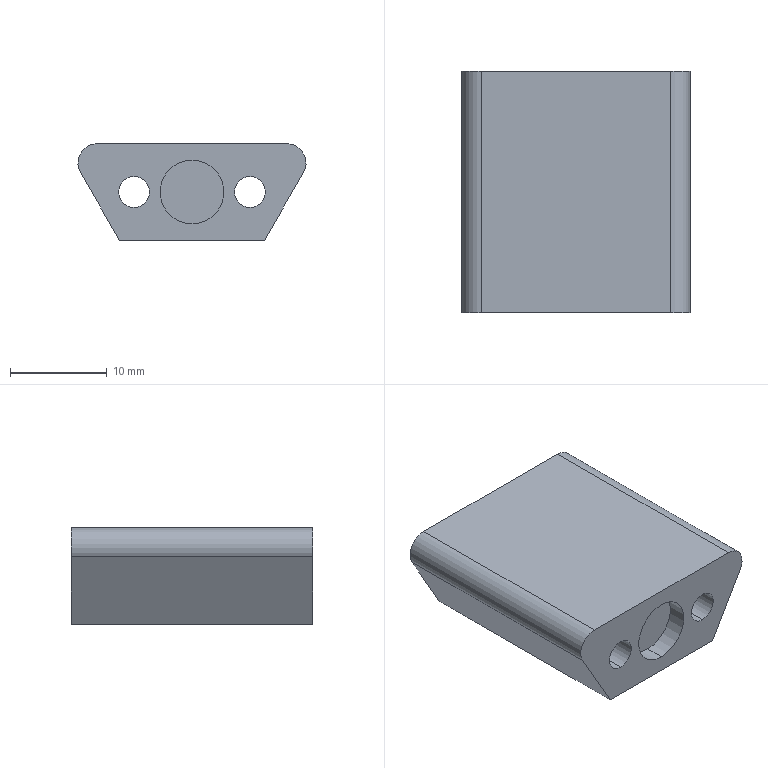Part | SolidWorks | features HoleWzd 2, ICE 2, Extrusion 1 | 1 solid | 29 faces | box 23.619 x 25 x 10 mm | volume 4394 mm3 | cylinder 16 | plane 9 | cone 4 | commonest cylinder face diameters 2.5 x4 3.2 x4 5 x4 4 x2 6.6 x2
STEP:
#1=CARTESIAN_POINT('',(13.274,-10.5,-1.7));
#2=VERTEX_POINT('',#1);
#3=CARTESIAN_POINT('',(13.274,-10.5,-8.3));
#4=VERTEX_POINT('',#3);
#5=CARTESIAN_POINT('',(13.274,-10.5,-5.));
#6=DIRECTION('',(0.,-1.,0.));
#7=DIRECTION('',(0.,0.,-1.));
#8=AXIS2_PLACEMENT_3D('',#5,#6,#7);
#9=CIRCLE('',#8,3.3);
#10=EDGE_CURVE('',#2,#4,#9,.T.);
#11=ORIENTED_EDGE('',*,*,#10,.F.);
#12=CARTESIAN_POINT('',(13.274,-12.5,-1.7));
#13=VERTEX_POINT('',#12);
#14=CARTESIAN_POINT('',(13.274,-10.5,-1.7));
#15=DIRECTION('',(0.,-1.,0.));
#16=VECTOR('',#15,1000.);
#17=LINE('',#14,#16);
#18=EDGE_CURVE('',#2,#13,#17,.T.);
#19=ORIENTED_EDGE('',*,*,#18,.T.);
#20=CARTESIAN_POINT('',(13.274,-12.5,-8.3));
#21=VERTEX_POINT('',#20);
#22=CARTESIAN_POINT('',(13.274,-12.5,-5.));
#23=DIRECTION('',(0.,-1.,0.));
#24=DIRECTION('',(0.,0.,-1.));
#25=AXIS2_PLACEMENT_3D('',#22,#23,#24);
#26=CIRCLE('',#25,3.3);
#27=EDGE_CURVE('',#13,#21,#26,.T.);
#28=ORIENTED_EDGE('',*,*,#27,.T.);
#29=CARTESIAN_POINT('',(13.274,-10.5,-8.3));
#30=DIRECTION('',(0.,-1.,0.));
#31=VECTOR('',#30,1000.);
#32=LINE('',#29,#31);
#33=EDGE_CURVE('',#4,#21,#32,.T.);
#34=ORIENTED_EDGE('',*,*,#33,.F.);
#35=EDGE_LOOP('',(#11,#19,#28,#34));
#36=FACE_OUTER_BOUND('',#35,.T.);
#37=CARTESIAN_POINT('',(13.274,-10.5,-5.));
#38=DIRECTION('',(0.,-1.,0.));
#39=DIRECTION('',(0.,0.,-1.));
#40=AXIS2_PLACEMENT_3D('',#37,#38,#39);
#41=CYLINDRICAL_SURFACE('',#40,3.3);
#42=ADVANCED_FACE('',(#36),#41,.F.);
#43=CARTESIAN_POINT('',(19.274,-12.5,-6.6));
#44=VERTEX_POINT('',#43);
#45=CARTESIAN_POINT('',(19.274,-12.5,-3.4));
#46=VERTEX_POINT('',#45);
#47=CARTESIAN_POINT('',(19.274,-12.5,-5.));
#48=DIRECTION('',(0.,1.,0.));
#49=DIRECTION('',(0.,0.,1.));
#50=AXIS2_PLACEMENT_3D('',#47,#48,#49);
#51=CIRCLE('',#50,1.6);
#52=EDGE_CURVE('',#44,#46,#51,.T.);
#53=ORIENTED_EDGE('',*,*,#52,.F.);
#54=CARTESIAN_POINT('',(19.274,7.5,-6.6));
#55=VERTEX_POINT('',#54);
#56=CARTESIAN_POINT('',(19.274,7.5,-6.6));
#57=DIRECTION('',(0.,1.,0.));
#58=VECTOR('',#57,1000.);
#59=LINE('',#56,#58);
#60=EDGE_CURVE('',#44,#55,#59,.T.);
#61=ORIENTED_EDGE('',*,*,#60,.T.);
#62=CARTESIAN_POINT('',(19.274,7.5,-3.4));
#63=VERTEX_POINT('',#62);
#64=CARTESIAN_POINT('',(19.274,7.5,-5.));
#65=DIRECTION('',(0.,1.,0.));
#66=DIRECTION('',(0.,0.,1.));
#67=AXIS2_PLACEMENT_3D('',#64,#65,#66);
#68=CIRCLE('',#67,1.6);
#69=EDGE_CURVE('',#55,#63,#68,.T.);
#70=ORIENTED_EDGE('',*,*,#69,.T.);
#71=CARTESIAN_POINT('',(19.274,7.5,-3.4));
#72=DIRECTION('',(0.,1.,0.));
#73=VECTOR('',#72,1000.);
#74=LINE('',#71,#73);
#75=EDGE_CURVE('',#46,#63,#74,.T.);
#76=ORIENTED_EDGE('',*,*,#75,.F.);
#77=EDGE_LOOP('',(#53,#61,#70,#76));
#78=FACE_OUTER_BOUND('',#77,.T.);
#79=CARTESIAN_POINT('',(19.274,7.5,-5.));
#80=DIRECTION('',(0.,1.,0.));
#81=DIRECTION('',(0.,0.,1.));
#82=AXIS2_PLACEMENT_3D('',#79,#80,#81);
#83=CYLINDRICAL_SURFACE('',#82,1.6);
#84=ADVANCED_FACE('',(#78),#83,.F.);
#85=CARTESIAN_POINT('',(7.274,-12.5,-6.6));
#86=VERTEX_POINT('',#85);
#87=CARTESIAN_POINT('',(7.274,-12.5,-3.4));
#88=VERTEX_POINT('',#87);
#89=CARTESIAN_POINT('',(7.274,-12.5,-5.));
#90=DIRECTION('',(0.,1.,0.));
#91=DIRECTION('',(0.,0.,1.));
#92=AXIS2_PLACEMENT_3D('',#89,#90,#91);
#93=CIRCLE('',#92,1.6);
#94=EDGE_CURVE('',#86,#88,#93,.T.);
#95=ORIENTED_EDGE('',*,*,#94,.F.);
#96=CARTESIAN_POINT('',(7.274,7.5,-6.6));
#97=VERTEX_POINT('',#96);
#98=CARTESIAN_POINT('',(7.274,7.5,-6.6));
#99=DIRECTION('',(0.,1.,0.));
#100=VECTOR('',#99,1000.);
#101=LINE('',#98,#100);
#102=EDGE_CURVE('',#86,#97,#101,.T.);
#103=ORIENTED_EDGE('',*,*,#102,.T.);
#104=CARTESIAN_POINT('',(7.274,7.5,-3.4));
#105=VERTEX_POINT('',#104);
#106=CARTESIAN_POINT('',(7.274,7.5,-5.));
#107=DIRECTION('',(0.,1.,0.));
#108=DIRECTION('',(0.,0.,1.));
#109=AXIS2_PLACEMENT_3D('',#106,#107,#108);
#110=CIRCLE('',#109,1.6);
#111=EDGE_CURVE('',#97,#105,#110,.T.);
#112=ORIENTED_EDGE('',*,*,#111,.T.);
#113=CARTESIAN_POINT('',(7.274,7.5,-3.4));
#114=DIRECTION('',(0.,1.,0.));
#115=VECTOR('',#114,1000.);
#116=LINE('',#113,#115);
#117=EDGE_CURVE('',#88,#105,#116,.T.);
#118=ORIENTED_EDGE('',*,*,#117,.F.);
#119=EDGE_LOOP('',(#95,#103,#112,#118));
#120=FACE_OUTER_BOUND('',#119,.T.);
#121=CARTESIAN_POINT('',(7.274,7.5,-5.));
#122=DIRECTION('',(0.,1.,0.));
#123=DIRECTION('',(0.,0.,1.));
#124=AXIS2_PLACEMENT_3D('',#121,#122,#123);
#125=CYLINDRICAL_SURFACE('',#124,1.6);
#126=ADVANCED_FACE('',(#120),#125,.F.);
#127=CARTESIAN_POINT('',(14.524,-5.,-2.5));
#128=VERTEX_POINT('',#127);
#129=CARTESIAN_POINT('',(12.024,-5.,-2.5));
#130=VERTEX_POINT('',#129);
#131=CARTESIAN_POINT('',(13.274,-5.,-2.5));
#132=DIRECTION('',(0.,0.,-1.));
#133=DIRECTION('',(-1.,0.,0.));
#134=AXIS2_PLACEMENT_3D('',#131,#132,#133);
#135=CIRCLE('',#134,1.25);
#136=EDGE_CURVE('',#128,#130,#135,.T.);
#137=ORIENTED_EDGE('',*,*,#136,.F.);
#138=CARTESIAN_POINT('',(14.524,-5.,-10.));
#139=VERTEX_POINT('',#138);
#140=CARTESIAN_POINT('',(14.524,-5.,-10.));
#141=DIRECTION('',(0.,0.,-1.));
#142=VECTOR('',#141,1000.);
#143=LINE('',#140,#142);
#144=EDGE_CURVE('',#128,#139,#143,.T.);
#145=ORIENTED_EDGE('',*,*,#144,.T.);
#146=CARTESIAN_POINT('',(12.024,-5.,-10.));
#147=VERTEX_POINT('',#146);
#148=CARTESIAN_POINT('',(13.274,-5.,-10.));
#149=DIRECTION('',(0.,0.,-1.));
#150=DIRECTION('',(-1.,0.,0.));
#151=AXIS2_PLACEMENT_3D('',#148,#149,#150);
#152=CIRCLE('',#151,1.25);
#153=EDGE_CURVE('',#139,#147,#152,.T.);
#154=ORIENTED_EDGE('',*,*,#153,.T.);
#155=CARTESIAN_POINT('',(12.024,-5.,-10.));
#156=DIRECTION('',(0.,0.,-1.));
#157=VECTOR('',#156,1000.);
#158=LINE('',#155,#157);
#159=EDGE_CURVE('',#130,#147,#158,.T.);
#160=ORIENTED_EDGE('',*,*,#159,.F.);
#161=EDGE_LOOP('',(#137,#145,#154,#160));
#162=FACE_OUTER_BOUND('',#161,.T.);
#163=CARTESIAN_POINT('',(13.274,-5.,-10.));
#164=DIRECTION('',(0.,0.,-1.));
#165=DIRECTION('',(-1.,0.,0.));
#166=AXIS2_PLACEMENT_3D('',#163,#164,#165);
#167=CYLINDRICAL_SURFACE('',#166,1.25);
#168=ADVANCED_FACE('',(#162),#167,.F.);
#169=CARTESIAN_POINT('',(13.274,-5.,-1.749));
#170=VERTEX_POINT('',#169);
#171=CARTESIAN_POINT('',(12.024,-5.,-2.5));
#172=DIRECTION('',(-0.8572,0.,-0.515));
#173=VECTOR('',#172,1000.);
#174=LINE('',#171,#173);
#175=EDGE_CURVE('',#170,#130,#174,.T.);
#176=ORIENTED_EDGE('',*,*,#175,.F.);
#177=CARTESIAN_POINT('',(14.524,-5.,-2.5));
#178=DIRECTION('',(0.8572,0.,-0.515));
#179=VECTOR('',#178,1000.);
#180=LINE('',#177,#179);
#181=EDGE_CURVE('',#170,#128,#180,.T.);
#182=ORIENTED_EDGE('',*,*,#181,.T.);
#183=ORIENTED_EDGE('',*,*,#136,.T.);
#184=EDGE_LOOP('',(#176,#182,#183));
#185=FACE_OUTER_BOUND('',#184,.T.);
#186=CARTESIAN_POINT('',(13.274,-5.,-2.5));
#187=DIRECTION('',(0.,0.,-1.));
#188=DIRECTION('',(-1.,0.,0.));
#189=AXIS2_PLACEMENT_3D('',#186,#187,#188);
#190=CONICAL_SURFACE('',#189,1.25,1.03);
#191=ADVANCED_FACE('',(#185),#190,.F.);
#192=CARTESIAN_POINT('',(14.524,5.,-2.5));
#193=VERTEX_POINT('',#192);
#194=CARTESIAN_POINT('',(12.024,5.,-2.5));
#195=VERTEX_POINT('',#194);
#196=CARTESIAN_POINT('',(13.274,5.,-2.5));
#197=DIRECTION('',(0.,0.,-1.));
#198=DIRECTION('',(-1.,0.,0.));
#199=AXIS2_PLACEMENT_3D('',#196,#197,#198);
#200=CIRCLE('',#199,1.25);
#201=EDGE_CURVE('',#193,#195,#200,.T.);
#202=ORIENTED_EDGE('',*,*,#201,.F.);
#203=CARTESIAN_POINT('',(14.524,5.,-10.));
#204=VERTEX_POINT('',#203);
#205=CARTESIAN_POINT('',(14.524,5.,-10.));
#206=DIRECTION('',(0.,0.,-1.));
#207=VECTOR('',#206,1000.);
#208=LINE('',#205,#207);
#209=EDGE_CURVE('',#193,#204,#208,.T.);
#210=ORIENTED_EDGE('',*,*,#209,.T.);
#211=CARTESIAN_POINT('',(12.024,5.,-10.));
#212=VERTEX_POINT('',#211);
#213=CARTESIAN_POINT('',(13.274,5.,-10.));
#214=DIRECTION('',(0.,0.,-1.));
#215=DIRECTION('',(-1.,0.,0.));
#216=AXIS2_PLACEMENT_3D('',#213,#214,#215);
#217=CIRCLE('',#216,1.25);
#218=EDGE_CURVE('',#204,#212,#217,.T.);
#219=ORIENTED_EDGE('',*,*,#218,.T.);
#220=CARTESIAN_POINT('',(12.024,5.,-10.));
#221=DIRECTION('',(0.,0.,-1.));
#222=VECTOR('',#221,1000.);
#223=LINE('',#220,#222);
#224=EDGE_CURVE('',#195,#212,#223,.T.);
#225=ORIENTED_EDGE('',*,*,#224,.F.);
#226=EDGE_LOOP('',(#202,#210,#219,#225));
#227=FACE_OUTER_BOUND('',#226,.T.);
#228=CARTESIAN_POINT('',(13.274,5.,-10.));
#229=DIRECTION('',(0.,0.,-1.));
#230=DIRECTION('',(-1.,0.,0.));
#231=AXIS2_PLACEMENT_3D('',#228,#229,#230);
#232=CYLINDRICAL_SURFACE('',#231,1.25);
#233=ADVANCED_FACE('',(#227),#232,.F.);
#234=CARTESIAN_POINT('',(13.274,5.,-1.749));
#235=VERTEX_POINT('',#234);
#236=CARTESIAN_POINT('',(12.024,5.,-2.5));
#237=DIRECTION('',(-0.8572,0.,-0.515));
#238=VECTOR('',#237,1000.);
#239=LINE('',#236,#238);
#240=EDGE_CURVE('',#235,#195,#239,.T.);
#241=ORIENTED_EDGE('',*,*,#240,.F.);
#242=CARTESIAN_POINT('',(14.524,5.,-2.5));
#243=DIRECTION('',(0.8572,0.,-0.515));
#244=VECTOR('',#243,1000.);
#245=LINE('',#242,#244);
#246=EDGE_CURVE('',#235,#193,#245,.T.);
#247=ORIENTED_EDGE('',*,*,#246,.T.);
#248=ORIENTED_EDGE('',*,*,#201,.T.);
#249=EDGE_LOOP('',(#241,#247,#248));
#250=FACE_OUTER_BOUND('',#249,.T.);
#251=CARTESIAN_POINT('',(13.274,5.,-2.5));
#252=DIRECTION('',(0.,0.,-1.));
#253=DIRECTION('',(-1.,0.,0.));
#254=AXIS2_PLACEMENT_3D('',#251,#252,#253);
#255=CONICAL_SURFACE('',#254,1.25,1.03);
#256=ADVANCED_FACE('',(#250),#255,.F.);
#257=CARTESIAN_POINT('',(19.274,7.5,-7.5));
#258=VERTEX_POINT('',#257);
#259=CARTESIAN_POINT('',(19.274,7.5,-2.5));
#260=VERTEX_POINT('',#259);
#261=CARTESIAN_POINT('',(19.274,7.5,-5.));
#262=DIRECTION('',(0.,1.,0.));
#263=DIRECTION('',(0.,0.,1.));
#264=AXIS2_PLACEMENT_3D('',#261,#262,#263);
#265=CIRCLE('',#264,2.5);
#266=EDGE_CURVE('',#258,#260,#265,.T.);
#267=ORIENTED_EDGE('',*,*,#266,.F.);
#268=CARTESIAN_POINT('',(19.274,12.5,-7.5));
#269=VERTEX_POINT('',#268);
#270=CARTESIAN_POINT('',(19.274,7.5,-7.5));
#271=DIRECTION('',(0.,1.,0.));
#272=VECTOR('',#271,1000.);
#273=LINE('',#270,#272);
#274=EDGE_CURVE('',#258,#269,#273,.T.);
#275=ORIENTED_EDGE('',*,*,#274,.T.);
#276=CARTESIAN_POINT('',(19.274,12.5,-2.5));
#277=VERTEX_POINT('',#276);
#278=CARTESIAN_POINT('',(19.274,12.5,-5.));
#279=DIRECTION('',(0.,1.,0.));
#280=DIRECTION('',(0.,0.,1.));
#281=AXIS2_PLACEMENT_3D('',#278,#279,#280);
#282=CIRCLE('',#281,2.5);
#283=EDGE_CURVE('',#269,#277,#282,.T.);
#284=ORIENTED_EDGE('',*,*,#283,.T.);
#285=CARTESIAN_POINT('',(19.274,7.5,-2.5));
#286=DIRECTION('',(0.,1.,0.));
#287=VECTOR('',#286,1000.);
#288=LINE('',#285,#287);
#289=EDGE_CURVE('',#260,#277,#288,.T.);
#290=ORIENTED_EDGE('',*,*,#289,.F.);
#291=EDGE_LOOP('',(#267,#275,#284,#290));
#292=FACE_OUTER_BOUND('',#291,.T.);
#293=CARTESIAN_POINT('',(19.274,7.5,-5.));
#294=DIRECTION('',(0.,1.,0.));
#295=DIRECTION('',(0.,0.,1.));
#296=AXIS2_PLACEMENT_3D('',#293,#294,#295);
#297=CYLINDRICAL_SURFACE('',#296,2.5);
#298=ADVANCED_FACE('',(#292),#297,.F.);
#299=CARTESIAN_POINT('',(7.274,7.5,-7.5));
#300=VERTEX_POINT('',#299);
#301=CARTESIAN_POINT('',(7.274,7.5,-2.5));
#302=VERTEX_POINT('',#301);
#303=CARTESIAN_POINT('',(7.274,7.5,-5.));
#304=DIRECTION('',(0.,1.,0.));
#305=DIRECTION('',(0.,0.,1.));
#306=AXIS2_PLACEMENT_3D('',#303,#304,#305);
#307=CIRCLE('',#306,2.5);
#308=EDGE_CURVE('',#300,#302,#307,.T.);
#309=ORIENTED_EDGE('',*,*,#308,.F.);
#310=CARTESIAN_POINT('',(7.274,12.5,-7.5));
#311=VERTEX_POINT('',#310);
#312=CARTESIAN_POINT('',(7.274,7.5,-7.5));
#313=DIRECTION('',(0.,1.,0.));
#314=VECTOR('',#313,1000.);
#315=LINE('',#312,#314);
#316=EDGE_CURVE('',#300,#311,#315,.T.);
#317=ORIENTED_EDGE('',*,*,#316,.T.);
#318=CARTESIAN_POINT('',(7.274,12.5,-2.5));
#319=VERTEX_POINT('',#318);
#320=CARTESIAN_POINT('',(7.274,12.5,-5.));
#321=DIRECTION('',(0.,1.,0.));
#322=DIRECTION('',(0.,0.,1.));
#323=AXIS2_PLACEMENT_3D('',#320,#321,#322);
#324=CIRCLE('',#323,2.5);
#325=EDGE_CURVE('',#311,#319,#324,.T.);
#326=ORIENTED_EDGE('',*,*,#325,.T.);
#327=CARTESIAN_POINT('',(7.274,7.5,-2.5));
#328=DIRECTION('',(0.,1.,0.));
#329=VECTOR('',#328,1000.);
#330=LINE('',#327,#329);
#331=EDGE_CURVE('',#302,#319,#330,.T.);
#332=ORIENTED_EDGE('',*,*,#331,.F.);
#333=EDGE_LOOP('',(#309,#317,#326,#332));
#334=FACE_OUTER_BOUND('',#333,.T.);
#335=CARTESIAN_POINT('',(7.274,7.5,-5.));
#336=DIRECTION('',(0.,1.,0.));
#337=DIRECTION('',(0.,0.,1.));
#338=AXIS2_PLACEMENT_3D('',#335,#336,#337);
#339=CYLINDRICAL_SURFACE('',#338,2.5);
#340=ADVANCED_FACE('',(#334),#339,.F.);
#341=CARTESIAN_POINT('',(13.274,-5.,-10.));
#342=DIRECTION('',(0.,0.,-1.));
#343=DIRECTION('',(-1.,0.,0.));
#344=AXIS2_PLACEMENT_3D('',#341,#342,#343);
#345=CIRCLE('',#344,1.25);
#346=EDGE_CURVE('',#147,#139,#345,.T.);
#347=ORIENTED_EDGE('',*,*,#346,.F.);
#348=ORIENTED_EDGE('',*,*,#153,.F.);
#349=EDGE_LOOP('',(#347,#348));
#350=FACE_BOUND('',#349,.T.);
#351=CARTESIAN_POINT('',(13.274,5.,-10.));
#352=DIRECTION('',(0.,0.,-1.));
#353=DIRECTION('',(-1.,0.,0.));
#354=AXIS2_PLACEMENT_3D('',#351,#352,#353);
#355=CIRCLE('',#354,1.25);
#356=EDGE_CURVE('',#212,#204,#355,.T.);
#357=ORIENTED_EDGE('',*,*,#356,.F.);
#358=ORIENTED_EDGE('',*,*,#218,.F.);
#359=EDGE_LOOP('',(#357,#358));
#360=FACE_BOUND('',#359,.T.);
#361=CARTESIAN_POINT('',(20.774,-12.5,-10.));
#362=VERTEX_POINT('',#361);
#363=CARTESIAN_POINT('',(5.774,-12.5,-10.));
#364=VERTEX_POINT('',#363);
#365=CARTESIAN_POINT('',(20.774,-12.5,-10.));
#366=DIRECTION('',(-1.,0.,0.));
#367=VECTOR('',#366,1000.);
#368=LINE('',#365,#367);
#369=EDGE_CURVE('',#362,#364,#368,.T.);
#370=ORIENTED_EDGE('',*,*,#369,.T.);
#371=CARTESIAN_POINT('',(5.774,12.5,-10.));
#372=VERTEX_POINT('',#371);
#373=CARTESIAN_POINT('',(5.774,12.5,-10.));
#374=DIRECTION('',(0.,-1.,0.));
#375=VECTOR('',#374,1000.);
#376=LINE('',#373,#375);
#377=EDGE_CURVE('',#372,#364,#376,.T.);
#378=ORIENTED_EDGE('',*,*,#377,.F.);
#379=CARTESIAN_POINT('',(20.774,12.5,-10.));
#380=VERTEX_POINT('',#379);
#381=CARTESIAN_POINT('',(20.774,12.5,-10.));
#382=DIRECTION('',(-1.,0.,0.));
#383=VECTOR('',#382,1000.);
#384=LINE('',#381,#383);
#385=EDGE_CURVE('',#380,#372,#384,.T.);
#386=ORIENTED_EDGE('',*,*,#385,.F.);
#387=CARTESIAN_POINT('',(20.774,12.5,-10.));
#388=DIRECTION('',(0.,-1.,0.));
#389=VECTOR('',#388,1000.);
#390=LINE('',#387,#389);
#391=EDGE_CURVE('',#380,#362,#390,.T.);
#392=ORIENTED_EDGE('',*,*,#391,.T.);
#393=EDGE_LOOP('',(#370,#378,#386,#392));
#394=FACE_OUTER_BOUND('',#393,.T.);
#395=CARTESIAN_POINT('',(20.774,12.5,-10.));
#396=DIRECTION('',(0.,0.,1.));
#397=DIRECTION('',(1.,0.,0.));
#398=AXIS2_PLACEMENT_3D('',#395,#396,#397);
#399=PLANE('',#398);
#400=ADVANCED_FACE('',(#350,#360,#394),#399,.F.);
#401=CARTESIAN_POINT('',(1.732,-12.5,-3.));
#402=VERTEX_POINT('',#401);
#403=CARTESIAN_POINT('',(5.774,-12.5,-10.));
#404=DIRECTION('',(-0.5,0.,0.866));
#405=VECTOR('',#404,1000.);
#406=LINE('',#403,#405);
#407=EDGE_CURVE('',#364,#402,#406,.T.);
#408=ORIENTED_EDGE('',*,*,#407,.T.);
#409=CARTESIAN_POINT('',(1.732,12.5,-3.));
#410=VERTEX_POINT('',#409);
#411=CARTESIAN_POINT('',(1.732,12.5,-3.));
#412=DIRECTION('',(0.,-1.,0.));
#413=VECTOR('',#412,1000.);
#414=LINE('',#411,#413);
#415=EDGE_CURVE('',#410,#402,#414,.T.);
#416=ORIENTED_EDGE('',*,*,#415,.F.);
#417=CARTESIAN_POINT('',(5.774,12.5,-10.));
#418=DIRECTION('',(-0.5,0.,0.866));
#419=VECTOR('',#418,1000.);
#420=LINE('',#417,#419);
#421=EDGE_CURVE('',#372,#410,#420,.T.);
#422=ORIENTED_EDGE('',*,*,#421,.F.);
#423=ORIENTED_EDGE('',*,*,#377,.T.);
#424=EDGE_LOOP('',(#408,#416,#422,#423));
#425=FACE_OUTER_BOUND('',#424,.T.);
#426=CARTESIAN_POINT('',(5.774,12.5,-10.));
#427=DIRECTION('',(0.866,0.,0.5));
#428=DIRECTION('',(0.5,0.,-0.866));
#429=AXIS2_PLACEMENT_3D('',#426,#427,#428);
#430=PLANE('',#429);
#431=ADVANCED_FACE('',(#425),#430,.F.);
#432=CARTESIAN_POINT('',(3.464,-12.5,0.));
#433=VERTEX_POINT('',#432);
#434=CARTESIAN_POINT('',(3.464,-12.5,-2.));
#435=DIRECTION('',(0.,1.,0.));
#436=DIRECTION('',(0.,0.,-1.));
#437=AXIS2_PLACEMENT_3D('',#434,#435,#436);
#438=CIRCLE('',#437,2.);
#439=EDGE_CURVE('',#402,#433,#438,.T.);
#440=ORIENTED_EDGE('',*,*,#439,.T.);
#441=CARTESIAN_POINT('',(3.464,12.5,0.));
#442=VERTEX_POINT('',#441);
#443=CARTESIAN_POINT('',(3.464,12.5,0.));
#444=DIRECTION('',(0.,-1.,0.));
#445=VECTOR('',#444,1000.);
#446=LINE('',#443,#445);
#447=EDGE_CURVE('',#442,#433,#446,.T.);
#448=ORIENTED_EDGE('',*,*,#447,.F.);
#449=CARTESIAN_POINT('',(3.464,12.5,-2.));
#450=DIRECTION('',(0.,1.,0.));
#451=DIRECTION('',(0.,0.,-1.));
#452=AXIS2_PLACEMENT_3D('',#449,#450,#451);
#453=CIRCLE('',#452,2.);
#454=EDGE_CURVE('',#410,#442,#453,.T.);
#455=ORIENTED_EDGE('',*,*,#454,.F.);
#456=ORIENTED_EDGE('',*,*,#415,.T.);
#457=EDGE_LOOP('',(#440,#448,#455,#456));
#458=FACE_OUTER_BOUND('',#457,.T.);
#459=CARTESIAN_POINT('',(3.464,12.5,-2.));
#460=DIRECTION('',(0.,-1.,0.));
#461=DIRECTION('',(0.,0.,-1.));
#462=AXIS2_PLACEMENT_3D('',#459,#460,#461);
#463=CYLINDRICAL_SURFACE('',#462,2.);
#464=ADVANCED_FACE('',(#458),#463,.T.);
#465=CARTESIAN_POINT('',(23.083,-12.5,0.));
#466=VERTEX_POINT('',#465);
#467=CARTESIAN_POINT('',(3.464,-12.5,0.));
#468=DIRECTION('',(1.,0.,0.));
#469=VECTOR('',#468,1000.);
#470=LINE('',#467,#469);
#471=EDGE_CURVE('',#433,#466,#470,.T.);
#472=ORIENTED_EDGE('',*,*,#471,.T.);
#473=CARTESIAN_POINT('',(23.083,12.5,0.));
#474=VERTEX_POINT('',#473);
#475=CARTESIAN_POINT('',(23.083,12.5,0.));
#476=DIRECTION('',(0.,-1.,0.));
#477=VECTOR('',#476,1000.);
#478=LINE('',#475,#477);
#479=EDGE_CURVE('',#474,#466,#478,.T.);
#480=ORIENTED_EDGE('',*,*,#479,.F.);
#481=CARTESIAN_POINT('',(3.464,12.5,0.));
#482=DIRECTION('',(1.,0.,0.));
#483=VECTOR('',#482,1000.);
#484=LINE('',#481,#483);
#485=EDGE_CURVE('',#442,#474,#484,.T.);
#486=ORIENTED_EDGE('',*,*,#485,.F.);
#487=ORIENTED_EDGE('',*,*,#447,.T.);
#488=EDGE_LOOP('',(#472,#480,#486,#487));
#489=FACE_OUTER_BOUND('',#488,.T.);
#490=CARTESIAN_POINT('',(3.464,12.5,0.));
#491=DIRECTION('',(0.,0.,-1.));
#492=DIRECTION('',(-1.,0.,0.));
#493=AXIS2_PLACEMENT_3D('',#490,#491,#492);
#494=PLANE('',#493);
#495=ADVANCED_FACE('',(#489),#494,.F.);
#496=CARTESIAN_POINT('',(24.815,-12.5,-3.));
#497=VERTEX_POINT('',#496);
#498=CARTESIAN_POINT('',(23.083,-12.5,-2.));
#499=DIRECTION('',(0.,1.,0.));
#500=DIRECTION('',(0.,0.,1.));
#501=AXIS2_PLACEMENT_3D('',#498,#499,#500);
#502=CIRCLE('',#501,2.);
#503=EDGE_CURVE('',#466,#497,#502,.T.);
#504=ORIENTED_EDGE('',*,*,#503,.T.);
#505=CARTESIAN_POINT('',(24.815,12.5,-3.));
#506=VERTEX_POINT('',#505);
#507=CARTESIAN_POINT('',(24.815,12.5,-3.));
#508=DIRECTION('',(0.,-1.,0.));
#509=VECTOR('',#508,1000.);
#510=LINE('',#507,#509);
#511=EDGE_CURVE('',#506,#497,#510,.T.);
#512=ORIENTED_EDGE('',*,*,#511,.F.);
#513=CARTESIAN_POINT('',(23.083,12.5,-2.));
#514=DIRECTION('',(0.,1.,0.));
#515=DIRECTION('',(0.,0.,1.));
#516=AXIS2_PLACEMENT_3D('',#513,#514,#515);
#517=CIRCLE('',#516,2.);
#518=EDGE_CURVE('',#474,#506,#517,.T.);
#519=ORIENTED_EDGE('',*,*,#518,.F.);
#520=ORIENTED_EDGE('',*,*,#479,.T.);
#521=EDGE_LOOP('',(#504,#512,#519,#520));
#522=FACE_OUTER_BOUND('',#521,.T.);
#523=CARTESIAN_POINT('',(23.083,12.5,-2.));
#524=DIRECTION('',(0.,-1.,0.));
#525=DIRECTION('',(0.,0.,-1.));
#526=AXIS2_PLACEMENT_3D('',#523,#524,#525);
#527=CYLINDRICAL_SURFACE('',#526,2.);
#528=ADVANCED_FACE('',(#522),#527,.T.);
#529=CARTESIAN_POINT('',(24.815,-12.5,-3.));
#530=DIRECTION('',(-0.5,0.,-0.866));
#531=VECTOR('',#530,1000.);
#532=LINE('',#529,#531);
#533=EDGE_CURVE('',#497,#362,#532,.T.);
#534=ORIENTED_EDGE('',*,*,#533,.T.);
#535=ORIENTED_EDGE('',*,*,#391,.F.);
#536=CARTESIAN_POINT('',(24.815,12.5,-3.));
#537=DIRECTION('',(-0.5,0.,-0.866));
#538=VECTOR('',#537,1000.);
#539=LINE('',#536,#538);
#540=EDGE_CURVE('',#506,#380,#539,.T.);
#541=ORIENTED_EDGE('',*,*,#540,.F.);
#542=ORIENTED_EDGE('',*,*,#511,.T.);
#543=EDGE_LOOP('',(#534,#535,#541,#542));
#544=FACE_OUTER_BOUND('',#543,.T.);
#545=CARTESIAN_POINT('',(24.815,12.5,-3.));
#546=DIRECTION('',(-0.866,0.,0.5));
#547=DIRECTION('',(0.5,0.,0.866));
#548=AXIS2_PLACEMENT_3D('',#545,#546,#547);
#549=PLANE('',#548);
#550=ADVANCED_FACE('',(#544),#549,.F.);
#551=CARTESIAN_POINT('',(19.274,12.5,-5.));
#552=DIRECTION('',(0.,1.,0.));
#553=DIRECTION('',(0.,0.,1.));
#554=AXIS2_PLACEMENT_3D('',#551,#552,#553);
#555=CIRCLE('',#554,2.5);
#556=EDGE_CURVE('',#277,#269,#555,.T.);
#557=ORIENTED_EDGE('',*,*,#556,.F.);
#558=ORIENTED_EDGE('',*,*,#283,.F.);
#559=EDGE_LOOP('',(#557,#558));
#560=FACE_BOUND('',#559,.T.);
#561=CARTESIAN_POINT('',(7.274,12.5,-5.));
#562=DIRECTION('',(0.,1.,0.));
#563=DIRECTION('',(0.,0.,1.));
#564=AXIS2_PLACEMENT_3D('',#561,#562,#563);
#565=CIRCLE('',#564,2.5);
#566=EDGE_CURVE('',#319,#311,#565,.T.);
#567=ORIENTED_EDGE('',*,*,#566,.F.);
#568=ORIENTED_EDGE('',*,*,#325,.F.);
#569=EDGE_LOOP('',(#567,#568));
#570=FACE_BOUND('',#569,.T.);
#571=ORIENTED_EDGE('',*,*,#385,.T.);
#572=ORIENTED_EDGE('',*,*,#421,.T.);
#573=ORIENTED_EDGE('',*,*,#454,.T.);
#574=ORIENTED_EDGE('',*,*,#485,.T.);
#575=ORIENTED_EDGE('',*,*,#518,.T.);
#576=ORIENTED_EDGE('',*,*,#540,.T.);
#577=EDGE_LOOP('',(#571,#572,#573,#574,#575,#576));
#578=FACE_OUTER_BOUND('',#577,.T.);
#579=CARTESIAN_POINT('',(3.464,12.5,-2.));
#580=DIRECTION('',(0.,-1.,0.));
#581=DIRECTION('',(0.,0.,-1.));
#582=AXIS2_PLACEMENT_3D('',#579,#580,#581);
#583=PLANE('',#582);
#584=ADVANCED_FACE('',(#560,#570,#578),#583,.F.);
#585=CARTESIAN_POINT('',(13.274,-12.5,-5.));
#586=DIRECTION('',(0.,-1.,0.));
#587=DIRECTION('',(0.,0.,-1.));
#588=AXIS2_PLACEMENT_3D('',#585,#586,#587);
#589=CIRCLE('',#588,3.3);
#590=EDGE_CURVE('',#21,#13,#589,.T.);
#591=ORIENTED_EDGE('',*,*,#590,.F.);
#592=ORIENTED_EDGE('',*,*,#27,.F.);
#593=EDGE_LOOP('',(#591,#592));
#594=FACE_BOUND('',#593,.T.);
#595=CARTESIAN_POINT('',(19.274,-12.5,-5.));
#596=DIRECTION('',(0.,1.,0.));
#597=DIRECTION('',(0.,0.,1.));
#598=AXIS2_PLACEMENT_3D('',#595,#596,#597);
#599=CIRCLE('',#598,1.6);
#600=EDGE_CURVE('',#46,#44,#599,.T.);
#601=ORIENTED_EDGE('',*,*,#600,.T.);
#602=ORIENTED_EDGE('',*,*,#52,.T.);
#603=EDGE_LOOP('',(#601,#602));
#604=FACE_BOUND('',#603,.T.);
#605=CARTESIAN_POINT('',(7.274,-12.5,-5.));
#606=DIRECTION('',(0.,1.,0.));
#607=DIRECTION('',(0.,0.,1.));
#608=AXIS2_PLACEMENT_3D('',#605,#606,#607);
#609=CIRCLE('',#608,1.6);
#610=EDGE_CURVE('',#88,#86,#609,.T.);
#611=ORIENTED_EDGE('',*,*,#610,.T.);
#612=ORIENTED_EDGE('',*,*,#94,.T.);
#613=EDGE_LOOP('',(#611,#612));
#614=FACE_BOUND('',#613,.T.);
#615=ORIENTED_EDGE('',*,*,#369,.F.);
#616=ORIENTED_EDGE('',*,*,#533,.F.);
#617=ORIENTED_EDGE('',*,*,#503,.F.);
#618=ORIENTED_EDGE('',*,*,#471,.F.);
#619=ORIENTED_EDGE('',*,*,#439,.F.);
#620=ORIENTED_EDGE('',*,*,#407,.F.);
#621=EDGE_LOOP('',(#615,#616,#617,#618,#619,#620));
#622=FACE_OUTER_BOUND('',#621,.T.);
#623=CARTESIAN_POINT('',(3.464,-12.5,-2.));
#624=DIRECTION('',(0.,-1.,0.));
#625=DIRECTION('',(0.,0.,-1.));
#626=AXIS2_PLACEMENT_3D('',#623,#624,#625);
#627=PLANE('',#626);
#628=ADVANCED_FACE('',(#594,#604,#614,#622),#627,.T.);
#629=ORIENTED_EDGE('',*,*,#316,.F.);
#630=CARTESIAN_POINT('',(7.274,7.5,-5.));
#631=DIRECTION('',(0.,1.,0.));
#632=DIRECTION('',(0.,0.,1.));
#633=AXIS2_PLACEMENT_3D('',#630,#631,#632);
#634=CIRCLE('',#633,2.5);
#635=EDGE_CURVE('',#302,#300,#634,.T.);
#636=ORIENTED_EDGE('',*,*,#635,.F.);
#637=ORIENTED_EDGE('',*,*,#331,.T.);
#638=ORIENTED_EDGE('',*,*,#566,.T.);
#639=EDGE_LOOP('',(#629,#636,#637,#638));
#640=FACE_OUTER_BOUND('',#639,.T.);
#641=CARTESIAN_POINT('',(7.274,7.5,-5.));
#642=DIRECTION('',(0.,1.,0.));
#643=DIRECTION('',(0.,0.,1.));
#644=AXIS2_PLACEMENT_3D('',#641,#642,#643);
#645=CYLINDRICAL_SURFACE('',#644,2.5);
#646=ADVANCED_FACE('',(#640),#645,.F.);
#647=CARTESIAN_POINT('',(7.274,7.5,-5.));
#648=DIRECTION('',(0.,1.,0.));
#649=DIRECTION('',(0.,0.,1.));
#650=AXIS2_PLACEMENT_3D('',#647,#648,#649);
#651=CIRCLE('',#650,1.6);
#652=EDGE_CURVE('',#105,#97,#651,.T.);
#653=ORIENTED_EDGE('',*,*,#652,.F.);
#654=ORIENTED_EDGE('',*,*,#111,.F.);
#655=EDGE_LOOP('',(#653,#654));
#656=FACE_BOUND('',#655,.T.);
#657=ORIENTED_EDGE('',*,*,#635,.T.);
#658=ORIENTED_EDGE('',*,*,#308,.T.);
#659=EDGE_LOOP('',(#657,#658));
#660=FACE_OUTER_BOUND('',#659,.T.);
#661=CARTESIAN_POINT('',(7.274,7.5,-5.));
#662=DIRECTION('',(0.,1.,0.));
#663=DIRECTION('',(0.,0.,1.));
#664=AXIS2_PLACEMENT_3D('',#661,#662,#663);
#665=PLANE('',#664);
#666=ADVANCED_FACE('',(#656,#660),#665,.T.);
#667=ORIENTED_EDGE('',*,*,#274,.F.);
#668=CARTESIAN_POINT('',(19.274,7.5,-5.));
#669=DIRECTION('',(0.,1.,0.));
#670=DIRECTION('',(0.,0.,1.));
#671=AXIS2_PLACEMENT_3D('',#668,#669,#670);
#672=CIRCLE('',#671,2.5);
#673=EDGE_CURVE('',#260,#258,#672,.T.);
#674=ORIENTED_EDGE('',*,*,#673,.F.);
#675=ORIENTED_EDGE('',*,*,#289,.T.);
#676=ORIENTED_EDGE('',*,*,#556,.T.);
#677=EDGE_LOOP('',(#667,#674,#675,#676));
#678=FACE_OUTER_BOUND('',#677,.T.);
#679=CARTESIAN_POINT('',(19.274,7.5,-5.));
#680=DIRECTION('',(0.,1.,0.));
#681=DIRECTION('',(0.,0.,1.));
#682=AXIS2_PLACEMENT_3D('',#679,#680,#681);
#683=CYLINDRICAL_SURFACE('',#682,2.5);
#684=ADVANCED_FACE('',(#678),#683,.F.);
#685=CARTESIAN_POINT('',(19.274,7.5,-5.));
#686=DIRECTION('',(0.,1.,0.));
#687=DIRECTION('',(0.,0.,1.));
#688=AXIS2_PLACEMENT_3D('',#685,#686,#687);
#689=CIRCLE('',#688,1.6);
#690=EDGE_CURVE('',#63,#55,#689,.T.);
#691=ORIENTED_EDGE('',*,*,#690,.F.);
#692=ORIENTED_EDGE('',*,*,#69,.F.);
#693=EDGE_LOOP('',(#691,#692));
#694=FACE_BOUND('',#693,.T.);
#695=ORIENTED_EDGE('',*,*,#673,.T.);
#696=ORIENTED_EDGE('',*,*,#266,.T.);
#697=EDGE_LOOP('',(#695,#696));
#698=FACE_OUTER_BOUND('',#697,.T.);
#699=CARTESIAN_POINT('',(19.274,7.5,-5.));
#700=DIRECTION('',(0.,1.,0.));
#701=DIRECTION('',(0.,0.,1.));
#702=AXIS2_PLACEMENT_3D('',#699,#700,#701);
#703=PLANE('',#702);
#704=ADVANCED_FACE('',(#694,#698),#703,.T.);
#705=ORIENTED_EDGE('',*,*,#246,.F.);
#706=ORIENTED_EDGE('',*,*,#240,.T.);
#707=CARTESIAN_POINT('',(13.274,5.,-2.5));
#708=DIRECTION('',(0.,0.,-1.));
#709=DIRECTION('',(-1.,0.,0.));
#710=AXIS2_PLACEMENT_3D('',#707,#708,#709);
#711=CIRCLE('',#710,1.25);
#712=EDGE_CURVE('',#195,#193,#711,.T.);
#713=ORIENTED_EDGE('',*,*,#712,.T.);
#714=EDGE_LOOP('',(#705,#706,#713));
#715=FACE_OUTER_BOUND('',#714,.T.);
#716=CARTESIAN_POINT('',(13.274,5.,-2.5));
#717=DIRECTION('',(0.,0.,-1.));
#718=DIRECTION('',(-1.,0.,0.));
#719=AXIS2_PLACEMENT_3D('',#716,#717,#718);
#720=CONICAL_SURFACE('',#719,1.25,1.03);
#721=ADVANCED_FACE('',(#715),#720,.F.);
#722=ORIENTED_EDGE('',*,*,#209,.F.);
#723=ORIENTED_EDGE('',*,*,#712,.F.);
#724=ORIENTED_EDGE('',*,*,#224,.T.);
#725=ORIENTED_EDGE('',*,*,#356,.T.);
#726=EDGE_LOOP('',(#722,#723,#724,#725));
#727=FACE_OUTER_BOUND('',#726,.T.);
#728=CARTESIAN_POINT('',(13.274,5.,-10.));
#729=DIRECTION('',(0.,0.,-1.));
#730=DIRECTION('',(-1.,0.,0.));
#731=AXIS2_PLACEMENT_3D('',#728,#729,#730);
#732=CYLINDRICAL_SURFACE('',#731,1.25);
#733=ADVANCED_FACE('',(#727),#732,.F.);
#734=ORIENTED_EDGE('',*,*,#181,.F.);
#735=ORIENTED_EDGE('',*,*,#175,.T.);
#736=CARTESIAN_POINT('',(13.274,-5.,-2.5));
#737=DIRECTION('',(0.,0.,-1.));
#738=DIRECTION('',(-1.,0.,0.));
#739=AXIS2_PLACEMENT_3D('',#736,#737,#738);
#740=CIRCLE('',#739,1.25);
#741=EDGE_CURVE('',#130,#128,#740,.T.);
#742=ORIENTED_EDGE('',*,*,#741,.T.);
#743=EDGE_LOOP('',(#734,#735,#742));
#744=FACE_OUTER_BOUND('',#743,.T.);
#745=CARTESIAN_POINT('',(13.274,-5.,-2.5));
#746=DIRECTION('',(0.,0.,-1.));
#747=DIRECTION('',(-1.,0.,0.));
#748=AXIS2_PLACEMENT_3D('',#745,#746,#747);
#749=CONICAL_SURFACE('',#748,1.25,1.03);
#750=ADVANCED_FACE('',(#744),#749,.F.);
#751=ORIENTED_EDGE('',*,*,#144,.F.);
#752=ORIENTED_EDGE('',*,*,#741,.F.);
#753=ORIENTED_EDGE('',*,*,#159,.T.);
#754=ORIENTED_EDGE('',*,*,#346,.T.);
#755=EDGE_LOOP('',(#751,#752,#753,#754));
#756=FACE_OUTER_BOUND('',#755,.T.);
#757=CARTESIAN_POINT('',(13.274,-5.,-10.));
#758=DIRECTION('',(0.,0.,-1.));
#759=DIRECTION('',(-1.,0.,0.));
#760=AXIS2_PLACEMENT_3D('',#757,#758,#759);
#761=CYLINDRICAL_SURFACE('',#760,1.25);
#762=ADVANCED_FACE('',(#756),#761,.F.);
#763=ORIENTED_EDGE('',*,*,#102,.F.);
#764=ORIENTED_EDGE('',*,*,#610,.F.);
#765=ORIENTED_EDGE('',*,*,#117,.T.);
#766=ORIENTED_EDGE('',*,*,#652,.T.);
#767=EDGE_LOOP('',(#763,#764,#765,#766));
#768=FACE_OUTER_BOUND('',#767,.T.);
#769=CARTESIAN_POINT('',(7.274,7.5,-5.));
#770=DIRECTION('',(0.,1.,0.));
#771=DIRECTION('',(0.,0.,1.));
#772=AXIS2_PLACEMENT_3D('',#769,#770,#771);
#773=CYLINDRICAL_SURFACE('',#772,1.6);
#774=ADVANCED_FACE('',(#768),#773,.F.);
#775=ORIENTED_EDGE('',*,*,#60,.F.);
#776=ORIENTED_EDGE('',*,*,#600,.F.);
#777=ORIENTED_EDGE('',*,*,#75,.T.);
#778=ORIENTED_EDGE('',*,*,#690,.T.);
#779=EDGE_LOOP('',(#775,#776,#777,#778));
#780=FACE_OUTER_BOUND('',#779,.T.);
#781=CARTESIAN_POINT('',(19.274,7.5,-5.));
#782=DIRECTION('',(0.,1.,0.));
#783=DIRECTION('',(0.,0.,1.));
#784=AXIS2_PLACEMENT_3D('',#781,#782,#783);
#785=CYLINDRICAL_SURFACE('',#784,1.6);
#786=ADVANCED_FACE('',(#780),#785,.F.);
#787=ORIENTED_EDGE('',*,*,#18,.F.);
#788=CARTESIAN_POINT('',(13.274,-10.5,-5.));
#789=DIRECTION('',(0.,-1.,0.));
#790=DIRECTION('',(0.,0.,-1.));
#791=AXIS2_PLACEMENT_3D('',#788,#789,#790);
#792=CIRCLE('',#791,3.3);
#793=EDGE_CURVE('',#4,#2,#792,.T.);
#794=ORIENTED_EDGE('',*,*,#793,.F.);
#795=ORIENTED_EDGE('',*,*,#33,.T.);
#796=ORIENTED_EDGE('',*,*,#590,.T.);
#797=EDGE_LOOP('',(#787,#794,#795,#796));
#798=FACE_OUTER_BOUND('',#797,.T.);
#799=CARTESIAN_POINT('',(13.274,-10.5,-5.));
#800=DIRECTION('',(0.,-1.,0.));
#801=DIRECTION('',(0.,0.,-1.));
#802=AXIS2_PLACEMENT_3D('',#799,#800,#801);
#803=CYLINDRICAL_SURFACE('',#802,3.3);
#804=ADVANCED_FACE('',(#798),#803,.F.);
#805=ORIENTED_EDGE('',*,*,#793,.T.);
#806=ORIENTED_EDGE('',*,*,#10,.T.);
#807=EDGE_LOOP('',(#805,#806));
#808=FACE_OUTER_BOUND('',#807,.T.);
#809=CARTESIAN_POINT('',(13.274,-10.5,-5.));
#810=DIRECTION('',(0.,-1.,0.));
#811=DIRECTION('',(0.,0.,-1.));
#812=AXIS2_PLACEMENT_3D('',#809,#810,#811);
#813=PLANE('',#812);
#814=ADVANCED_FACE('',(#808),#813,.T.);
#815=CLOSED_SHELL('',(#42,#84,#126,#168,#191,#233,#256,#298,#340,#400,#431,#464,#495,#528,#550,#584,#628,#646,#666,#684,#704,#721,#733,#750,#762,#774,#786,#804,#814));
#816=MANIFOLD_SOLID_BREP('',#815);
#817=CARTESIAN_POINT('',(0.,0.,0.));
#818=DIRECTION('',(0.,0.,1.));
#819=DIRECTION('',(1.,0.,0.));
#820=AXIS2_PLACEMENT_3D('',#817,#818,#819);
#821=(LENGTH_UNIT()NAMED_UNIT(*)SI_UNIT(.MILLI.,.METRE.));
#822=UNCERTAINTY_MEASURE_WITH_UNIT(LENGTH_MEASURE(0.00001),#821,'','');
#823=(NAMED_UNIT(*)PLANE_ANGLE_UNIT()SI_UNIT($,.RADIAN.));
#824=(NAMED_UNIT(*)SI_UNIT($,.STERADIAN.)SOLID_ANGLE_UNIT());
#825=(GEOMETRIC_REPRESENTATION_CONTEXT(3)GLOBAL_UNCERTAINTY_ASSIGNED_CONTEXT((#822))GLOBAL_UNIT_ASSIGNED_CONTEXT((#821,#823,#824))REPRESENTATION_CONTEXT('',''));
#826=ADVANCED_BREP_SHAPE_REPRESENTATION('',(#816,#820),#825);